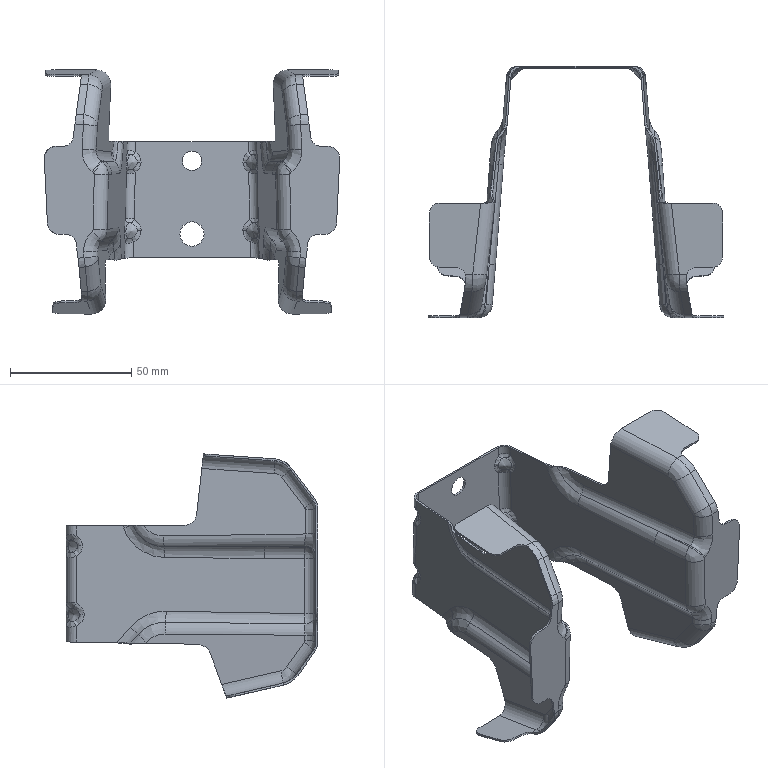Part | STEP file | FNA5401991 | 1 solid | 332 faces | box 121.896 x 103.862 x 100.696 mm | volume 16854 mm3 | spline 199 | cylinder 86 | plane 43 | other 4 | commonest cylinder face diameters 10 x22 11.6 x16 12 x12 7.4 x6 9 x6 10.4 x6